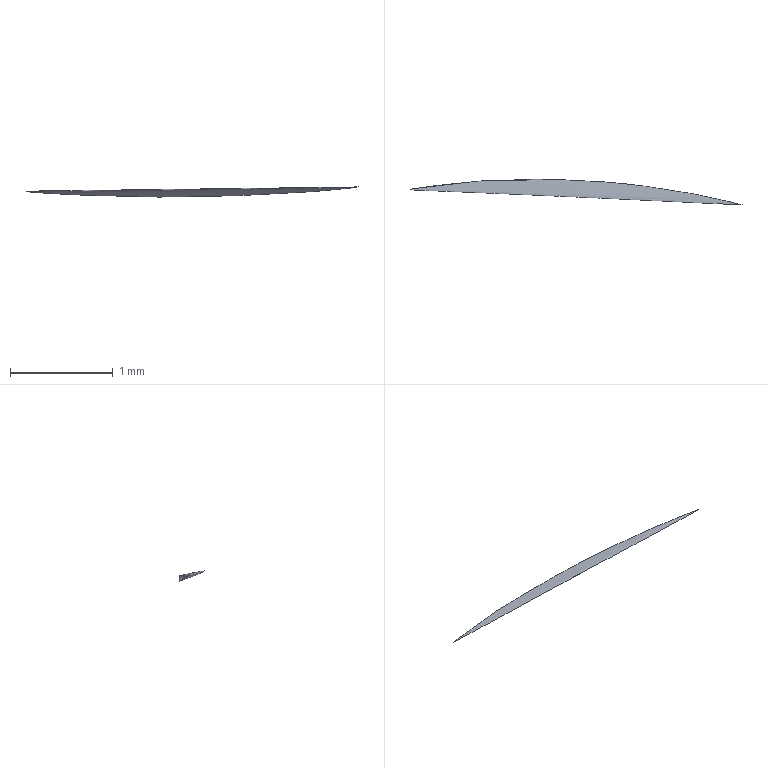Part | NX | features solid 2 | 1 solid | 2 faces | box 3.263 x 0.2526 x 0.09895 mm | volume 0.008156 mm3 | spline 1 | cylinder 1 | commonest cylinder face diameters 16 x1